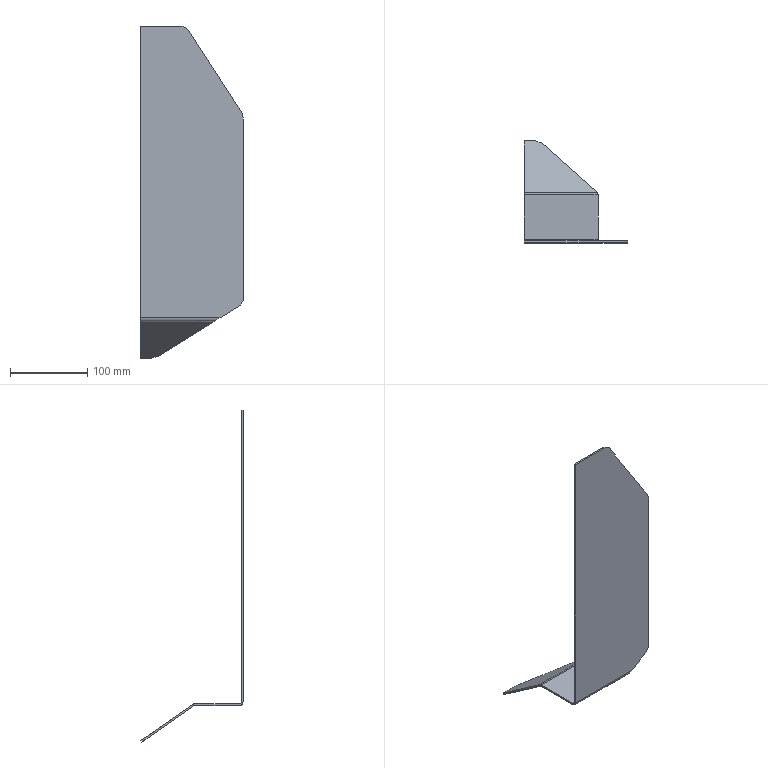Part | SolidWorks | features Chamfer 1, FlatPattern 1, ICE 1, SMBaseFlange 1, SheetMetal 1 | 1 solid | 28 faces | box 134 x 132 x 429.026 mm | volume 130634 mm3 | plane 22 | cylinder 4 | spline 2 | commonest cylinder face diameters 5 x2 9.6 x2
STEP:
#1=CARTESIAN_POINT('',(-52.,128.384,-429.026));
#2=VERTEX_POINT('',#1);
#3=CARTESIAN_POINT('',(-67.,128.384,-429.026));
#4=VERTEX_POINT('',#3);
#5=CARTESIAN_POINT('',(67.,128.384,-429.026));
#6=DIRECTION('',(-1.,0.,0.));
#7=VECTOR('',#6,1000.);
#8=LINE('',#5,#7);
#9=EDGE_CURVE('',#2,#4,#8,.T.);
#10=ORIENTED_EDGE('',*,*,#9,.F.);
#11=CARTESIAN_POINT('',(-43.618,125.364,-426.919));
#12=VERTEX_POINT('',#11);
#13=CARTESIAN_POINT('',(-43.618,125.364,-426.919));
#14=DIRECTION('',(0.9155,-0.3299,0.2302));
#15=VECTOR('',#14,1000.);
#16=LINE('',#13,#15);
#17=EDGE_CURVE('',#2,#12,#16,.T.);
#18=ORIENTED_EDGE('',*,*,#17,.T.);
#19=CARTESIAN_POINT('',(27.757,61.622,-382.45));
#20=VERTEX_POINT('',#19);
#21=CARTESIAN_POINT('',(46.463,44.916,-370.795));
#22=DIRECTION('',(0.6764,-0.6041,0.4214));
#23=VECTOR('',#22,1000.);
#24=LINE('',#21,#23);
#25=EDGE_CURVE('',#12,#20,#24,.T.);
#26=ORIENTED_EDGE('',*,*,#25,.T.);
#27=CARTESIAN_POINT('',(-67.,61.622,-382.45));
#28=VERTEX_POINT('',#27);
#29=CARTESIAN_POINT('',(67.,61.622,-382.45));
#30=DIRECTION('',(-1.,0.,0.));
#31=VECTOR('',#30,1000.);
#32=LINE('',#29,#31);
#33=EDGE_CURVE('',#20,#28,#32,.T.);
#34=ORIENTED_EDGE('',*,*,#33,.T.);
#35=CARTESIAN_POINT('',(-67.,60.384,-381.586));
#36=DIRECTION('',(0.,0.8201,-0.5722));
#37=VECTOR('',#36,1000.);
#38=LINE('',#35,#37);
#39=EDGE_CURVE('',#28,#4,#38,.T.);
#40=ORIENTED_EDGE('',*,*,#39,.T.);
#41=EDGE_LOOP('',(#10,#18,#26,#34,#40));
#42=FACE_OUTER_BOUND('',#41,.T.);
#43=CARTESIAN_POINT('',(67.,60.384,-381.586));
#44=DIRECTION('',(0.,0.5722,0.8201));
#45=DIRECTION('',(0.,-0.8201,0.5722));
#46=AXIS2_PLACEMENT_3D('',#43,#44,#45);
#47=PLANE('',#46);
#48=ADVANCED_FACE('',(#42),#47,.F.);
#49=CARTESIAN_POINT('',(-52.,129.7,-427.14));
#50=VERTEX_POINT('',#49);
#51=CARTESIAN_POINT('',(-67.,129.7,-427.14));
#52=VERTEX_POINT('',#51);
#53=CARTESIAN_POINT('',(67.,129.7,-427.14));
#54=DIRECTION('',(-1.,0.,0.));
#55=VECTOR('',#54,1000.);
#56=LINE('',#53,#55);
#57=EDGE_CURVE('',#50,#52,#56,.T.);
#58=ORIENTED_EDGE('',*,*,#57,.F.);
#59=CARTESIAN_POINT('',(-52.,129.7,-427.14));
#60=DIRECTION('',(0.,-0.5722,-0.8201));
#61=VECTOR('',#60,1000.);
#62=LINE('',#59,#61);
#63=EDGE_CURVE('',#50,#2,#62,.T.);
#64=ORIENTED_EDGE('',*,*,#63,.T.);
#65=ORIENTED_EDGE('',*,*,#9,.T.);
#66=CARTESIAN_POINT('',(-67.,129.7,-427.14));
#67=DIRECTION('',(0.,-0.5722,-0.8201));
#68=VECTOR('',#67,1000.);
#69=LINE('',#66,#68);
#70=EDGE_CURVE('',#52,#4,#69,.T.);
#71=ORIENTED_EDGE('',*,*,#70,.F.);
#72=EDGE_LOOP('',(#58,#64,#65,#71));
#73=FACE_OUTER_BOUND('',#72,.T.);
#74=CARTESIAN_POINT('',(67.,129.7,-427.14));
#75=DIRECTION('',(0.,0.8201,-0.5722));
#76=DIRECTION('',(0.,0.5722,0.8201));
#77=AXIS2_PLACEMENT_3D('',#74,#75,#76);
#78=PLANE('',#77);
#79=ADVANCED_FACE('',(#73),#78,.T.);
#80=CARTESIAN_POINT('',(-43.618,126.68,-425.033));
#81=VERTEX_POINT('',#80);
#82=CARTESIAN_POINT('',(27.757,62.938,-380.563));
#83=VERTEX_POINT('',#82);
#84=CARTESIAN_POINT('',(46.463,46.232,-368.909));
#85=DIRECTION('',(0.6764,-0.6041,0.4214));
#86=VECTOR('',#85,1000.);
#87=LINE('',#84,#86);
#88=EDGE_CURVE('',#81,#83,#87,.T.);
#89=ORIENTED_EDGE('',*,*,#88,.F.);
#90=CARTESIAN_POINT('',(78.28,82.756,-394.39));
#91=DIRECTION('',(-0.9155,0.3299,-0.2302));
#92=VECTOR('',#91,1000.);
#93=LINE('',#90,#92);
#94=EDGE_CURVE('',#81,#50,#93,.T.);
#95=ORIENTED_EDGE('',*,*,#94,.T.);
#96=ORIENTED_EDGE('',*,*,#57,.T.);
#97=CARTESIAN_POINT('',(-67.,62.938,-380.563));
#98=VERTEX_POINT('',#97);
#99=CARTESIAN_POINT('',(-67.,61.7,-379.7));
#100=DIRECTION('',(0.,0.8201,-0.5722));
#101=VECTOR('',#100,1000.);
#102=LINE('',#99,#101);
#103=EDGE_CURVE('',#98,#52,#102,.T.);
#104=ORIENTED_EDGE('',*,*,#103,.F.);
#105=CARTESIAN_POINT('',(67.,62.938,-380.563));
#106=DIRECTION('',(-1.,0.,0.));
#107=VECTOR('',#106,1000.);
#108=LINE('',#105,#107);
#109=EDGE_CURVE('',#83,#98,#108,.T.);
#110=ORIENTED_EDGE('',*,*,#109,.F.);
#111=EDGE_LOOP('',(#89,#95,#96,#104,#110));
#112=FACE_OUTER_BOUND('',#111,.T.);
#113=CARTESIAN_POINT('',(67.,61.7,-379.7));
#114=DIRECTION('',(0.,0.5722,0.8201));
#115=DIRECTION('',(0.,-0.8201,0.5722));
#116=AXIS2_PLACEMENT_3D('',#113,#114,#115);
#117=PLANE('',#116);
#118=ADVANCED_FACE('',(#112),#117,.T.);
#119=CARTESIAN_POINT('',(28.479,60.191,-379.7));
#120=VERTEX_POINT('',#119);
#121=CARTESIAN_POINT('',(-67.,60.191,-379.7));
#122=VERTEX_POINT('',#121);
#123=CARTESIAN_POINT('',(67.,60.191,-379.7));
#124=DIRECTION('',(-1.,0.,0.));
#125=VECTOR('',#124,1000.);
#126=LINE('',#123,#125);
#127=EDGE_CURVE('',#120,#122,#126,.T.);
#128=ORIENTED_EDGE('',*,*,#127,.F.);
#129=CARTESIAN_POINT('',(27.757,62.938,-380.563));
#130=CARTESIAN_POINT('',(28.231,62.126,-379.997));
#131=CARTESIAN_POINT('',(28.479,61.181,-379.7));
#132=CARTESIAN_POINT('',(28.479,60.191,-379.7));
#133=(BOUNDED_CURVE()B_SPLINE_CURVE(3,(#129,#130,#131,#132),.UNSPECIFIED.,.F.,.F.)B_SPLINE_CURVE_WITH_KNOTS((4,4),(2.532,3.142),.UNSPECIFIED.)CURVE()GEOMETRIC_REPRESENTATION_ITEM()RATIONAL_B_SPLINE_CURVE((1.,0.9693,0.9693,1.))REPRESENTATION_ITEM(''));
#134=EDGE_CURVE('',#83,#120,#133,.T.);
#135=ORIENTED_EDGE('',*,*,#134,.F.);
#136=ORIENTED_EDGE('',*,*,#109,.T.);
#137=CARTESIAN_POINT('',(-67.,60.191,-384.5));
#138=DIRECTION('',(-1.,0.,0.));
#139=DIRECTION('',(0.,0.,-1.));
#140=AXIS2_PLACEMENT_3D('',#137,#138,#139);
#141=CIRCLE('',#140,4.8);
#142=EDGE_CURVE('',#122,#98,#141,.T.);
#143=ORIENTED_EDGE('',*,*,#142,.F.);
#144=EDGE_LOOP('',(#128,#135,#136,#143));
#145=FACE_OUTER_BOUND('',#144,.T.);
#146=CARTESIAN_POINT('',(67.,60.191,-384.5));
#147=DIRECTION('',(-1.,0.,0.));
#148=DIRECTION('',(0.,0.,1.));
#149=AXIS2_PLACEMENT_3D('',#146,#147,#148);
#150=CYLINDRICAL_SURFACE('',#149,4.8);
#151=ADVANCED_FACE('',(#145),#150,.T.);
#152=CARTESIAN_POINT('',(28.479,2.5,-379.7));
#153=VERTEX_POINT('',#152);
#154=CARTESIAN_POINT('',(-67.,2.5,-379.7));
#155=VERTEX_POINT('',#154);
#156=CARTESIAN_POINT('',(67.,2.5,-379.7));
#157=DIRECTION('',(-1.,0.,0.));
#158=VECTOR('',#157,1000.);
#159=LINE('',#156,#158);
#160=EDGE_CURVE('',#153,#155,#159,.T.);
#161=ORIENTED_EDGE('',*,*,#160,.F.);
#162=CARTESIAN_POINT('',(28.479,0.,-379.7));
#163=DIRECTION('',(0.,-1.,0.));
#164=VECTOR('',#163,1000.);
#165=LINE('',#162,#164);
#166=EDGE_CURVE('',#120,#153,#165,.T.);
#167=ORIENTED_EDGE('',*,*,#166,.F.);
#168=ORIENTED_EDGE('',*,*,#127,.T.);
#169=CARTESIAN_POINT('',(-67.,0.,-379.7));
#170=DIRECTION('',(0.,1.,0.));
#171=VECTOR('',#170,1000.);
#172=LINE('',#169,#171);
#173=EDGE_CURVE('',#155,#122,#172,.T.);
#174=ORIENTED_EDGE('',*,*,#173,.F.);
#175=EDGE_LOOP('',(#161,#167,#168,#174));
#176=FACE_OUTER_BOUND('',#175,.T.);
#177=CARTESIAN_POINT('',(67.,0.,-379.7));
#178=DIRECTION('',(0.,0.,1.));
#179=DIRECTION('',(1.,0.,0.));
#180=AXIS2_PLACEMENT_3D('',#177,#178,#179);
#181=PLANE('',#180);
#182=ADVANCED_FACE('',(#176),#181,.T.);
#183=CARTESIAN_POINT('',(36.183,0.,-377.2));
#184=VERTEX_POINT('',#183);
#185=CARTESIAN_POINT('',(-67.,0.,-377.2));
#186=VERTEX_POINT('',#185);
#187=CARTESIAN_POINT('',(67.,0.,-377.2));
#188=DIRECTION('',(-1.,0.,0.));
#189=VECTOR('',#188,1000.);
#190=LINE('',#187,#189);
#191=EDGE_CURVE('',#184,#186,#190,.T.);
#192=ORIENTED_EDGE('',*,*,#191,.F.);
#193=CARTESIAN_POINT('',(28.479,2.5,-379.7));
#194=CARTESIAN_POINT('',(28.479,1.036,-379.7));
#195=CARTESIAN_POINT('',(31.67,0.,-378.664));
#196=CARTESIAN_POINT('',(36.183,0.,-377.2));
#197=(BOUNDED_CURVE()B_SPLINE_CURVE(3,(#193,#194,#195,#196),.UNSPECIFIED.,.F.,.T.)B_SPLINE_CURVE_WITH_KNOTS((4,4),(0.,1.571),.UNSPECIFIED.)CURVE()GEOMETRIC_REPRESENTATION_ITEM()RATIONAL_B_SPLINE_CURVE((1.,0.8047,0.8047,1.))REPRESENTATION_ITEM(''));
#198=EDGE_CURVE('',#153,#184,#197,.T.);
#199=ORIENTED_EDGE('',*,*,#198,.F.);
#200=ORIENTED_EDGE('',*,*,#160,.T.);
#201=CARTESIAN_POINT('',(-67.,2.5,-377.2));
#202=DIRECTION('',(1.,0.,0.));
#203=DIRECTION('',(0.,0.,1.));
#204=AXIS2_PLACEMENT_3D('',#201,#202,#203);
#205=CIRCLE('',#204,2.5);
#206=EDGE_CURVE('',#186,#155,#205,.T.);
#207=ORIENTED_EDGE('',*,*,#206,.F.);
#208=EDGE_LOOP('',(#192,#199,#200,#207));
#209=FACE_OUTER_BOUND('',#208,.T.);
#210=CARTESIAN_POINT('',(67.,2.5,-377.2));
#211=DIRECTION('',(-1.,0.,0.));
#212=DIRECTION('',(0.,0.,1.));
#213=AXIS2_PLACEMENT_3D('',#210,#211,#212);
#214=CYLINDRICAL_SURFACE('',#213,2.5);
#215=ADVANCED_FACE('',(#209),#214,.F.);
#216=CARTESIAN_POINT('',(67.,0.,-121.5));
#217=VERTEX_POINT('',#216);
#218=CARTESIAN_POINT('',(67.,0.,-353.));
#219=VERTEX_POINT('',#218);
#220=CARTESIAN_POINT('',(67.,0.,0.));
#221=DIRECTION('',(0.,0.,-1.));
#222=VECTOR('',#221,1000.);
#223=LINE('',#220,#222);
#224=EDGE_CURVE('',#217,#219,#223,.T.);
#225=ORIENTED_EDGE('',*,*,#224,.T.);
#226=CARTESIAN_POINT('',(62.756,0.,-360.644));
#227=VERTEX_POINT('',#226);
#228=CARTESIAN_POINT('',(216.804,0.,-83.167));
#229=DIRECTION('',(-0.4854,0.,-0.8743));
#230=VECTOR('',#229,1000.);
#231=LINE('',#228,#230);
#232=EDGE_CURVE('',#219,#227,#231,.T.);
#233=ORIENTED_EDGE('',*,*,#232,.T.);
#234=CARTESIAN_POINT('',(227.677,0.,-257.892));
#235=DIRECTION('',(0.8487,0.,0.5288));
#236=VECTOR('',#235,1000.);
#237=LINE('',#234,#236);
#238=EDGE_CURVE('',#184,#227,#237,.T.);
#239=ORIENTED_EDGE('',*,*,#238,.F.);
#240=ORIENTED_EDGE('',*,*,#191,.T.);
#241=CARTESIAN_POINT('',(-67.,0.,0.));
#242=VERTEX_POINT('',#241);
#243=CARTESIAN_POINT('',(-67.,0.,0.));
#244=DIRECTION('',(0.,0.,-1.));
#245=VECTOR('',#244,1000.);
#246=LINE('',#243,#245);
#247=EDGE_CURVE('',#242,#186,#246,.T.);
#248=ORIENTED_EDGE('',*,*,#247,.F.);
#249=CARTESIAN_POINT('',(-13.,0.,0.));
#250=VERTEX_POINT('',#249);
#251=CARTESIAN_POINT('',(67.,0.,0.));
#252=DIRECTION('',(-1.,0.,0.));
#253=VECTOR('',#252,1000.);
#254=LINE('',#251,#253);
#255=EDGE_CURVE('',#250,#242,#254,.T.);
#256=ORIENTED_EDGE('',*,*,#255,.F.);
#257=CARTESIAN_POINT('',(-5.293,0.,-4.204));
#258=VERTEX_POINT('',#257);
#259=CARTESIAN_POINT('',(48.652,0.,-33.633));
#260=DIRECTION('',(0.8779,0.,-0.4789));
#261=VECTOR('',#260,1000.);
#262=LINE('',#259,#261);
#263=EDGE_CURVE('',#250,#258,#262,.T.);
#264=ORIENTED_EDGE('',*,*,#263,.T.);
#265=CARTESIAN_POINT('',(64.293,0.,-112.296));
#266=VERTEX_POINT('',#265);
#267=CARTESIAN_POINT('',(13.976,0.,-34.136));
#268=DIRECTION('',(-0.5413,0.,0.8408));
#269=VECTOR('',#268,1000.);
#270=LINE('',#267,#269);
#271=EDGE_CURVE('',#266,#258,#270,.T.);
#272=ORIENTED_EDGE('',*,*,#271,.F.);
#273=CARTESIAN_POINT('',(34.116,0.,-9.67));
#274=DIRECTION('',(0.2821,0.,-0.9594));
#275=VECTOR('',#274,1000.);
#276=LINE('',#273,#275);
#277=EDGE_CURVE('',#266,#217,#276,.T.);
#278=ORIENTED_EDGE('',*,*,#277,.T.);
#279=EDGE_LOOP('',(#225,#233,#239,#240,#248,#256,#264,#272,#278));
#280=FACE_OUTER_BOUND('',#279,.T.);
#281=CARTESIAN_POINT('',(67.,0.,0.));
#282=DIRECTION('',(0.,1.,0.));
#283=DIRECTION('',(0.,0.,1.));
#284=AXIS2_PLACEMENT_3D('',#281,#282,#283);
#285=PLANE('',#284);
#286=ADVANCED_FACE('',(#280),#285,.T.);
#287=CARTESIAN_POINT('',(-13.,-2.3,0.));
#288=VERTEX_POINT('',#287);
#289=CARTESIAN_POINT('',(-67.,-2.3,0.));
#290=VERTEX_POINT('',#289);
#291=CARTESIAN_POINT('',(67.,-2.3,0.));
#292=DIRECTION('',(-1.,0.,0.));
#293=VECTOR('',#292,1000.);
#294=LINE('',#291,#293);
#295=EDGE_CURVE('',#288,#290,#294,.T.);
#296=ORIENTED_EDGE('',*,*,#295,.F.);
#297=CARTESIAN_POINT('',(-13.,-2.3,0.));
#298=DIRECTION('',(0.,1.,0.));
#299=VECTOR('',#298,1000.);
#300=LINE('',#297,#299);
#301=EDGE_CURVE('',#288,#250,#300,.T.);
#302=ORIENTED_EDGE('',*,*,#301,.T.);
#303=ORIENTED_EDGE('',*,*,#255,.T.);
#304=CARTESIAN_POINT('',(-67.,-2.3,0.));
#305=DIRECTION('',(0.,1.,0.));
#306=VECTOR('',#305,1000.);
#307=LINE('',#304,#306);
#308=EDGE_CURVE('',#290,#242,#307,.T.);
#309=ORIENTED_EDGE('',*,*,#308,.F.);
#310=EDGE_LOOP('',(#296,#302,#303,#309));
#311=FACE_OUTER_BOUND('',#310,.T.);
#312=CARTESIAN_POINT('',(67.,-2.3,0.));
#313=DIRECTION('',(0.,0.,1.));
#314=DIRECTION('',(1.,0.,0.));
#315=AXIS2_PLACEMENT_3D('',#312,#313,#314);
#316=PLANE('',#315);
#317=ADVANCED_FACE('',(#311),#316,.T.);
#318=CARTESIAN_POINT('',(36.183,-2.3,-377.2));
#319=VERTEX_POINT('',#318);
#320=CARTESIAN_POINT('',(62.756,-2.3,-360.644));
#321=VERTEX_POINT('',#320);
#322=CARTESIAN_POINT('',(227.677,-2.3,-257.892));
#323=DIRECTION('',(0.8487,0.,0.5288));
#324=VECTOR('',#323,1000.);
#325=LINE('',#322,#324);
#326=EDGE_CURVE('',#319,#321,#325,.T.);
#327=ORIENTED_EDGE('',*,*,#326,.T.);
#328=CARTESIAN_POINT('',(67.,-2.3,-353.));
#329=VERTEX_POINT('',#328);
#330=CARTESIAN_POINT('',(62.756,-2.3,-360.644));
#331=DIRECTION('',(0.4854,0.,0.8743));
#332=VECTOR('',#331,1000.);
#333=LINE('',#330,#332);
#334=EDGE_CURVE('',#321,#329,#333,.T.);
#335=ORIENTED_EDGE('',*,*,#334,.T.);
#336=CARTESIAN_POINT('',(67.,-2.3,-121.5));
#337=VERTEX_POINT('',#336);
#338=CARTESIAN_POINT('',(67.,-2.3,0.));
#339=DIRECTION('',(0.,0.,-1.));
#340=VECTOR('',#339,1000.);
#341=LINE('',#338,#340);
#342=EDGE_CURVE('',#337,#329,#341,.T.);
#343=ORIENTED_EDGE('',*,*,#342,.F.);
#344=CARTESIAN_POINT('',(64.293,-2.3,-112.296));
#345=VERTEX_POINT('',#344);
#346=CARTESIAN_POINT('',(67.,-2.3,-121.5));
#347=DIRECTION('',(-0.2821,0.,0.9594));
#348=VECTOR('',#347,1000.);
#349=LINE('',#346,#348);
#350=EDGE_CURVE('',#337,#345,#349,.T.);
#351=ORIENTED_EDGE('',*,*,#350,.T.);
#352=CARTESIAN_POINT('',(-5.293,-2.3,-4.204));
#353=VERTEX_POINT('',#352);
#354=CARTESIAN_POINT('',(13.976,-2.3,-34.136));
#355=DIRECTION('',(-0.5413,0.,0.8408));
#356=VECTOR('',#355,1000.);
#357=LINE('',#354,#356);
#358=EDGE_CURVE('',#345,#353,#357,.T.);
#359=ORIENTED_EDGE('',*,*,#358,.T.);
#360=CARTESIAN_POINT('',(-5.293,-2.3,-4.204));
#361=DIRECTION('',(-0.8779,0.,0.4789));
#362=VECTOR('',#361,1000.);
#363=LINE('',#360,#362);
#364=EDGE_CURVE('',#353,#288,#363,.T.);
#365=ORIENTED_EDGE('',*,*,#364,.T.);
#366=ORIENTED_EDGE('',*,*,#295,.T.);
#367=CARTESIAN_POINT('',(-67.,-2.3,-377.2));
#368=VERTEX_POINT('',#367);
#369=CARTESIAN_POINT('',(-67.,-2.3,0.));
#370=DIRECTION('',(0.,0.,-1.));
#371=VECTOR('',#370,1000.);
#372=LINE('',#369,#371);
#373=EDGE_CURVE('',#290,#368,#372,.T.);
#374=ORIENTED_EDGE('',*,*,#373,.T.);
#375=CARTESIAN_POINT('',(67.,-2.3,-377.2));
#376=DIRECTION('',(-1.,0.,0.));
#377=VECTOR('',#376,1000.);
#378=LINE('',#375,#377);
#379=EDGE_CURVE('',#319,#368,#378,.T.);
#380=ORIENTED_EDGE('',*,*,#379,.F.);
#381=EDGE_LOOP('',(#327,#335,#343,#351,#359,#365,#366,#374,#380));
#382=FACE_OUTER_BOUND('',#381,.T.);
#383=CARTESIAN_POINT('',(67.,-2.3,0.));
#384=DIRECTION('',(0.,1.,0.));
#385=DIRECTION('',(0.,0.,1.));
#386=AXIS2_PLACEMENT_3D('',#383,#384,#385);
#387=PLANE('',#386);
#388=ADVANCED_FACE('',(#382),#387,.F.);
#389=CARTESIAN_POINT('',(28.479,2.5,-382.));
#390=VERTEX_POINT('',#389);
#391=CARTESIAN_POINT('',(28.479,2.5,-382.));
#392=CARTESIAN_POINT('',(28.479,-0.3118,-382.));
#393=CARTESIAN_POINT('',(31.67,-2.3,-380.012));
#394=CARTESIAN_POINT('',(36.183,-2.3,-377.2));
#395=(BOUNDED_CURVE()B_SPLINE_CURVE(3,(#391,#392,#393,#394),.UNSPECIFIED.,.F.,.F.)B_SPLINE_CURVE_WITH_KNOTS((4,4),(0.,1.571),.UNSPECIFIED.)CURVE()GEOMETRIC_REPRESENTATION_ITEM()RATIONAL_B_SPLINE_CURVE((1.,0.8047,0.8047,1.))REPRESENTATION_ITEM(''));
#396=EDGE_CURVE('',#390,#319,#395,.T.);
#397=ORIENTED_EDGE('',*,*,#396,.T.);
#398=ORIENTED_EDGE('',*,*,#379,.T.);
#399=CARTESIAN_POINT('',(-67.,2.5,-382.));
#400=VERTEX_POINT('',#399);
#401=CARTESIAN_POINT('',(-67.,2.5,-377.2));
#402=DIRECTION('',(1.,0.,0.));
#403=DIRECTION('',(0.,0.,-1.));
#404=AXIS2_PLACEMENT_3D('',#401,#402,#403);
#405=CIRCLE('',#404,4.8);
#406=EDGE_CURVE('',#368,#400,#405,.T.);
#407=ORIENTED_EDGE('',*,*,#406,.T.);
#408=CARTESIAN_POINT('',(67.,2.5,-382.));
#409=DIRECTION('',(-1.,0.,0.));
#410=VECTOR('',#409,1000.);
#411=LINE('',#408,#410);
#412=EDGE_CURVE('',#390,#400,#411,.T.);
#413=ORIENTED_EDGE('',*,*,#412,.F.);
#414=EDGE_LOOP('',(#397,#398,#407,#413));
#415=FACE_OUTER_BOUND('',#414,.T.);
#416=CARTESIAN_POINT('',(67.,2.5,-377.2));
#417=DIRECTION('',(-1.,0.,0.));
#418=DIRECTION('',(0.,0.,1.));
#419=AXIS2_PLACEMENT_3D('',#416,#417,#418);
#420=CYLINDRICAL_SURFACE('',#419,4.8);
#421=ADVANCED_FACE('',(#415),#420,.T.);
#422=CARTESIAN_POINT('',(28.479,60.191,-382.));
#423=VERTEX_POINT('',#422);
#424=CARTESIAN_POINT('',(28.479,0.,-382.));
#425=DIRECTION('',(0.,-1.,0.));
#426=VECTOR('',#425,1000.);
#427=LINE('',#424,#426);
#428=EDGE_CURVE('',#423,#390,#427,.T.);
#429=ORIENTED_EDGE('',*,*,#428,.T.);
#430=ORIENTED_EDGE('',*,*,#412,.T.);
#431=CARTESIAN_POINT('',(-67.,60.191,-382.));
#432=VERTEX_POINT('',#431);
#433=CARTESIAN_POINT('',(-67.,0.,-382.));
#434=DIRECTION('',(0.,1.,0.));
#435=VECTOR('',#434,1000.);
#436=LINE('',#433,#435);
#437=EDGE_CURVE('',#400,#432,#436,.T.);
#438=ORIENTED_EDGE('',*,*,#437,.T.);
#439=CARTESIAN_POINT('',(67.,60.191,-382.));
#440=DIRECTION('',(-1.,0.,0.));
#441=VECTOR('',#440,1000.);
#442=LINE('',#439,#441);
#443=EDGE_CURVE('',#423,#432,#442,.T.);
#444=ORIENTED_EDGE('',*,*,#443,.F.);
#445=EDGE_LOOP('',(#429,#430,#438,#444));
#446=FACE_OUTER_BOUND('',#445,.T.);
#447=CARTESIAN_POINT('',(67.,0.,-382.));
#448=DIRECTION('',(0.,0.,1.));
#449=DIRECTION('',(1.,0.,0.));
#450=AXIS2_PLACEMENT_3D('',#447,#448,#449);
#451=PLANE('',#450);
#452=ADVANCED_FACE('',(#446),#451,.F.);
#453=CARTESIAN_POINT('',(27.757,61.622,-382.45));
#454=CARTESIAN_POINT('',(28.231,61.199,-382.155));
#455=CARTESIAN_POINT('',(28.479,60.707,-382.));
#456=CARTESIAN_POINT('',(28.479,60.191,-382.));
#457=(BOUNDED_CURVE()B_SPLINE_CURVE(3,(#453,#454,#455,#456),.UNSPECIFIED.,.F.,.T.)B_SPLINE_CURVE_WITH_KNOTS((4,4),(2.532,3.142),.UNSPECIFIED.)CURVE()GEOMETRIC_REPRESENTATION_ITEM()RATIONAL_B_SPLINE_CURVE((1.,0.9693,0.9693,1.))REPRESENTATION_ITEM(''));
#458=EDGE_CURVE('',#20,#423,#457,.T.);
#459=ORIENTED_EDGE('',*,*,#458,.T.);
#460=ORIENTED_EDGE('',*,*,#443,.T.);
#461=CARTESIAN_POINT('',(-67.,60.191,-384.5));
#462=DIRECTION('',(-1.,0.,0.));
#463=DIRECTION('',(0.,0.,-1.));
#464=AXIS2_PLACEMENT_3D('',#461,#462,#463);
#465=CIRCLE('',#464,2.5);
#466=EDGE_CURVE('',#432,#28,#465,.T.);
#467=ORIENTED_EDGE('',*,*,#466,.T.);
#468=ORIENTED_EDGE('',*,*,#33,.F.);
#469=EDGE_LOOP('',(#459,#460,#467,#468));
#470=FACE_OUTER_BOUND('',#469,.T.);
#471=CARTESIAN_POINT('',(67.,60.191,-384.5));
#472=DIRECTION('',(-1.,0.,0.));
#473=DIRECTION('',(0.,0.,1.));
#474=AXIS2_PLACEMENT_3D('',#471,#472,#473);
#475=CYLINDRICAL_SURFACE('',#474,2.5);
#476=ADVANCED_FACE('',(#470),#475,.F.);
#477=ORIENTED_EDGE('',*,*,#342,.T.);
#478=CARTESIAN_POINT('',(67.,60.191,-353.));
#479=DIRECTION('',(0.,1.,0.));
#480=VECTOR('',#479,1000.);
#481=LINE('',#478,#480);
#482=EDGE_CURVE('',#329,#219,#481,.T.);
#483=ORIENTED_EDGE('',*,*,#482,.T.);
#484=ORIENTED_EDGE('',*,*,#224,.F.);
#485=CARTESIAN_POINT('',(67.,60.191,-121.5));
#486=DIRECTION('',(0.,-1.,0.));
#487=VECTOR('',#486,1000.);
#488=LINE('',#485,#487);
#489=EDGE_CURVE('',#217,#337,#488,.T.);
#490=ORIENTED_EDGE('',*,*,#489,.T.);
#491=EDGE_LOOP('',(#477,#483,#484,#490));
#492=FACE_OUTER_BOUND('',#491,.T.);
#493=CARTESIAN_POINT('',(67.,60.191,-384.5));
#494=DIRECTION('',(1.,0.,0.));
#495=DIRECTION('',(0.,0.,-1.));
#496=AXIS2_PLACEMENT_3D('',#493,#494,#495);
#497=PLANE('',#496);
#498=ADVANCED_FACE('',(#492),#497,.T.);
#499=CARTESIAN_POINT('',(-67.,0.,-377.2));
#500=DIRECTION('',(0.,-1.,0.));
#501=VECTOR('',#500,1000.);
#502=LINE('',#499,#501);
#503=EDGE_CURVE('',#186,#368,#502,.T.);
#504=ORIENTED_EDGE('',*,*,#503,.F.);
#505=ORIENTED_EDGE('',*,*,#206,.T.);
#506=CARTESIAN_POINT('',(-67.,2.5,-382.));
#507=DIRECTION('',(0.,0.,1.));
#508=VECTOR('',#507,1000.);
#509=LINE('',#506,#508);
#510=EDGE_CURVE('',#400,#155,#509,.T.);
#511=ORIENTED_EDGE('',*,*,#510,.F.);
#512=ORIENTED_EDGE('',*,*,#406,.F.);
#513=EDGE_LOOP('',(#504,#505,#511,#512));
#514=FACE_OUTER_BOUND('',#513,.T.);
#515=CARTESIAN_POINT('',(-67.,0.,-377.2));
#516=DIRECTION('',(-1.,0.,0.));
#517=DIRECTION('',(0.,0.,1.));
#518=AXIS2_PLACEMENT_3D('',#515,#516,#517);
#519=PLANE('',#518);
#520=ADVANCED_FACE('',(#514),#519,.T.);
#521=ORIENTED_EDGE('',*,*,#247,.T.);
#522=ORIENTED_EDGE('',*,*,#503,.T.);
#523=ORIENTED_EDGE('',*,*,#373,.F.);
#524=ORIENTED_EDGE('',*,*,#308,.T.);
#525=EDGE_LOOP('',(#521,#522,#523,#524));
#526=FACE_OUTER_BOUND('',#525,.T.);
#527=CARTESIAN_POINT('',(-67.,2.5,-382.));
#528=DIRECTION('',(-1.,0.,0.));
#529=DIRECTION('',(0.,0.,1.));
#530=AXIS2_PLACEMENT_3D('',#527,#528,#529);
#531=PLANE('',#530);
#532=ADVANCED_FACE('',(#526),#531,.T.);
#533=CARTESIAN_POINT('',(-67.,60.191,-379.7));
#534=DIRECTION('',(0.,0.,-1.));
#535=VECTOR('',#534,1000.);
#536=LINE('',#533,#535);
#537=EDGE_CURVE('',#122,#432,#536,.T.);
#538=ORIENTED_EDGE('',*,*,#537,.F.);
#539=ORIENTED_EDGE('',*,*,#142,.T.);
#540=CARTESIAN_POINT('',(-67.,61.622,-382.45));
#541=DIRECTION('',(0.,0.5722,0.8201));
#542=VECTOR('',#541,1000.);
#543=LINE('',#540,#542);
#544=EDGE_CURVE('',#28,#98,#543,.T.);
#545=ORIENTED_EDGE('',*,*,#544,.F.);
#546=ORIENTED_EDGE('',*,*,#466,.F.);
#547=EDGE_LOOP('',(#538,#539,#545,#546));
#548=FACE_OUTER_BOUND('',#547,.T.);
#549=CARTESIAN_POINT('',(-67.,60.191,-379.7));
#550=DIRECTION('',(-1.,0.,0.));
#551=DIRECTION('',(0.,0.,1.));
#552=AXIS2_PLACEMENT_3D('',#549,#550,#551);
#553=PLANE('',#552);
#554=ADVANCED_FACE('',(#548),#553,.T.);
#555=ORIENTED_EDGE('',*,*,#173,.T.);
#556=ORIENTED_EDGE('',*,*,#537,.T.);
#557=ORIENTED_EDGE('',*,*,#437,.F.);
#558=ORIENTED_EDGE('',*,*,#510,.T.);
#559=EDGE_LOOP('',(#555,#556,#557,#558));
#560=FACE_OUTER_BOUND('',#559,.T.);
#561=CARTESIAN_POINT('',(-67.,61.622,-382.45));
#562=DIRECTION('',(-1.,0.,0.));
#563=DIRECTION('',(0.,0.,1.));
#564=AXIS2_PLACEMENT_3D('',#561,#562,#563);
#565=PLANE('',#564);
#566=ADVANCED_FACE('',(#560),#565,.T.);
#567=ORIENTED_EDGE('',*,*,#39,.F.);
#568=ORIENTED_EDGE('',*,*,#544,.T.);
#569=ORIENTED_EDGE('',*,*,#103,.T.);
#570=ORIENTED_EDGE('',*,*,#70,.T.);
#571=EDGE_LOOP('',(#567,#568,#569,#570));
#572=FACE_OUTER_BOUND('',#571,.T.);
#573=CARTESIAN_POINT('',(-67.,60.191,-384.5));
#574=DIRECTION('',(1.,0.,0.));
#575=DIRECTION('',(0.,0.,-1.));
#576=AXIS2_PLACEMENT_3D('',#573,#574,#575);
#577=PLANE('',#576);
#578=ADVANCED_FACE('',(#572),#577,.F.);
#579=CARTESIAN_POINT('',(28.479,2.5,-382.));
#580=DIRECTION('',(0.,0.,1.));
#581=VECTOR('',#580,1000.);
#582=LINE('',#579,#581);
#583=EDGE_CURVE('',#390,#153,#582,.T.);
#584=ORIENTED_EDGE('',*,*,#583,.F.);
#585=ORIENTED_EDGE('',*,*,#428,.F.);
#586=CARTESIAN_POINT('',(28.479,60.191,-382.));
#587=DIRECTION('',(0.,0.,1.));
#588=VECTOR('',#587,1000.);
#589=LINE('',#586,#588);
#590=EDGE_CURVE('',#423,#120,#589,.T.);
#591=ORIENTED_EDGE('',*,*,#590,.T.);
#592=ORIENTED_EDGE('',*,*,#166,.T.);
#593=EDGE_LOOP('',(#584,#585,#591,#592));
#594=FACE_OUTER_BOUND('',#593,.T.);
#595=CARTESIAN_POINT('',(28.479,0.,-382.));
#596=DIRECTION('',(-1.,0.,0.));
#597=DIRECTION('',(0.,-1.,0.));
#598=AXIS2_PLACEMENT_3D('',#595,#596,#597);
#599=PLANE('',#598);
#600=ADVANCED_FACE('',(#594),#599,.F.);
#601=CARTESIAN_POINT('',(36.183,0.,-377.2));
#602=DIRECTION('',(0.,-1.,0.));
#603=VECTOR('',#602,1000.);
#604=LINE('',#601,#603);
#605=EDGE_CURVE('',#184,#319,#604,.T.);
#606=ORIENTED_EDGE('',*,*,#605,.T.);
#607=ORIENTED_EDGE('',*,*,#396,.F.);
#608=ORIENTED_EDGE('',*,*,#583,.T.);
#609=ORIENTED_EDGE('',*,*,#198,.T.);
#610=EDGE_LOOP('',(#606,#607,#608,#609));
#611=FACE_OUTER_BOUND('',#610,.T.);
#612=CARTESIAN_POINT('',(28.479,2.5,-379.7));
#613=CARTESIAN_POINT('',(28.479,2.5,-380.467));
#614=CARTESIAN_POINT('',(28.479,2.5,-381.233));
#615=CARTESIAN_POINT('',(28.479,2.5,-382.));
#616=CARTESIAN_POINT('',(28.479,-2.5,-379.7));
#617=CARTESIAN_POINT('',(28.479,-4.033,-380.467));
#618=CARTESIAN_POINT('',(28.479,-5.567,-381.233));
#619=CARTESIAN_POINT('',(28.479,-7.1,-382.));
#620=CARTESIAN_POINT('',(43.887,-2.5,-374.7));
#621=CARTESIAN_POINT('',(43.887,-4.033,-373.933));
#622=CARTESIAN_POINT('',(43.887,-5.567,-373.167));
#623=CARTESIAN_POINT('',(43.887,-7.1,-372.4));
#624=CARTESIAN_POINT('',(43.887,2.5,-374.7));
#625=CARTESIAN_POINT('',(43.887,2.5,-373.933));
#626=CARTESIAN_POINT('',(43.887,2.5,-373.167));
#627=CARTESIAN_POINT('',(43.887,2.5,-372.4));
#628=CARTESIAN_POINT('',(43.887,7.5,-374.7));
#629=CARTESIAN_POINT('',(43.887,9.033,-373.933));
#630=CARTESIAN_POINT('',(43.887,10.567,-373.167));
#631=CARTESIAN_POINT('',(43.887,12.1,-372.4));
#632=CARTESIAN_POINT('',(28.479,7.5,-379.7));
#633=CARTESIAN_POINT('',(28.479,9.033,-380.467));
#634=CARTESIAN_POINT('',(28.479,10.567,-381.233));
#635=CARTESIAN_POINT('',(28.479,12.1,-382.));
#636=CARTESIAN_POINT('',(28.479,2.5,-379.7));
#637=CARTESIAN_POINT('',(28.479,2.5,-380.467));
#638=CARTESIAN_POINT('',(28.479,2.5,-381.233));
#639=CARTESIAN_POINT('',(28.479,2.5,-382.));
#640=(BOUNDED_SURFACE()B_SPLINE_SURFACE(3,3,((#612,#613,#614,#615),(#616,#617,#618,#619),(#620,#621,#622,#623),(#624,#625,#626,#627),(#628,#629,#630,#631),(#632,#633,#634,#635),(#636,#637,#638,#639)),.UNSPECIFIED.,.T.,.F.,.T.)B_SPLINE_SURFACE_WITH_KNOTS((4,3,4),(4,4),(0.,0.5,1.),(0.,1.),.UNSPECIFIED.)GEOMETRIC_REPRESENTATION_ITEM()RATIONAL_B_SPLINE_SURFACE(((1.,1.,1.,1.),(0.3333,0.3333,0.3333,0.3333),(0.3333,0.3333,0.3333,0.3333),(1.,1.,1.,1.),(0.3333,0.3333,0.3333,0.3333),(0.3333,0.3333,0.3333,0.3333),(1.,1.,1.,1.)))REPRESENTATION_ITEM('')SURFACE());
#641=ADVANCED_FACE('',(#611),#640,.T.);
#642=ORIENTED_EDGE('',*,*,#238,.T.);
#643=CARTESIAN_POINT('',(62.756,0.,-360.644));
#644=DIRECTION('',(0.,-1.,0.));
#645=VECTOR('',#644,1000.);
#646=LINE('',#643,#645);
#647=EDGE_CURVE('',#227,#321,#646,.T.);
#648=ORIENTED_EDGE('',*,*,#647,.T.);
#649=ORIENTED_EDGE('',*,*,#326,.F.);
#650=ORIENTED_EDGE('',*,*,#605,.F.);
#651=EDGE_LOOP('',(#642,#648,#649,#650));
#652=FACE_OUTER_BOUND('',#651,.T.);
#653=CARTESIAN_POINT('',(227.677,0.,-257.892));
#654=DIRECTION('',(-0.5288,0.,0.8487));
#655=DIRECTION('',(0.8487,0.,0.5288));
#656=AXIS2_PLACEMENT_3D('',#653,#654,#655);
#657=PLANE('',#656);
#658=ADVANCED_FACE('',(#652),#657,.F.);
#659=ORIENTED_EDGE('',*,*,#590,.F.);
#660=ORIENTED_EDGE('',*,*,#458,.F.);
#661=CARTESIAN_POINT('',(27.757,61.622,-382.45));
#662=DIRECTION('',(0.,0.5722,0.8201));
#663=VECTOR('',#662,1000.);
#664=LINE('',#661,#663);
#665=EDGE_CURVE('',#20,#83,#664,.T.);
#666=ORIENTED_EDGE('',*,*,#665,.T.);
#667=ORIENTED_EDGE('',*,*,#134,.T.);
#668=EDGE_LOOP('',(#659,#660,#666,#667));
#669=FACE_OUTER_BOUND('',#668,.T.);
#670=CARTESIAN_POINT('',(20.454,60.191,-389.3));
#671=CARTESIAN_POINT('',(20.454,60.191,-388.533));
#672=CARTESIAN_POINT('',(20.454,60.191,-387.767));
#673=CARTESIAN_POINT('',(20.454,60.191,-387.));
#674=CARTESIAN_POINT('',(20.454,69.791,-389.3));
#675=CARTESIAN_POINT('',(20.454,68.258,-388.533));
#676=CARTESIAN_POINT('',(20.454,66.724,-387.767));
#677=CARTESIAN_POINT('',(20.454,65.191,-387.));
#678=CARTESIAN_POINT('',(28.479,69.791,-379.7));
#679=CARTESIAN_POINT('',(28.479,68.258,-380.467));
#680=CARTESIAN_POINT('',(28.479,66.724,-381.233));
#681=CARTESIAN_POINT('',(28.479,65.191,-382.));
#682=CARTESIAN_POINT('',(28.479,60.191,-379.7));
#683=CARTESIAN_POINT('',(28.479,60.191,-380.467));
#684=CARTESIAN_POINT('',(28.479,60.191,-381.233));
#685=CARTESIAN_POINT('',(28.479,60.191,-382.));
#686=CARTESIAN_POINT('',(28.479,50.591,-379.7));
#687=CARTESIAN_POINT('',(28.479,52.124,-380.467));
#688=CARTESIAN_POINT('',(28.479,53.658,-381.233));
#689=CARTESIAN_POINT('',(28.479,55.191,-382.));
#690=CARTESIAN_POINT('',(20.454,50.591,-389.3));
#691=CARTESIAN_POINT('',(20.454,52.124,-388.533));
#692=CARTESIAN_POINT('',(20.454,53.658,-387.767));
#693=CARTESIAN_POINT('',(20.454,55.191,-387.));
#694=CARTESIAN_POINT('',(20.454,60.191,-389.3));
#695=CARTESIAN_POINT('',(20.454,60.191,-388.533));
#696=CARTESIAN_POINT('',(20.454,60.191,-387.767));
#697=CARTESIAN_POINT('',(20.454,60.191,-387.));
#698=(BOUNDED_SURFACE()B_SPLINE_SURFACE(3,3,((#670,#671,#672,#673),(#674,#675,#676,#677),(#678,#679,#680,#681),(#682,#683,#684,#685),(#686,#687,#688,#689),(#690,#691,#692,#693),(#694,#695,#696,#697)),.UNSPECIFIED.,.T.,.F.,.T.)B_SPLINE_SURFACE_WITH_KNOTS((4,3,4),(4,4),(0.,0.5,1.),(0.,1.),.UNSPECIFIED.)GEOMETRIC_REPRESENTATION_ITEM()RATIONAL_B_SPLINE_SURFACE(((1.,1.,1.,1.),(0.3333,0.3333,0.3333,0.3333),(0.3333,0.3333,0.3333,0.3333),(1.,1.,1.,1.),(0.3333,0.3333,0.3333,0.3333),(0.3333,0.3333,0.3333,0.3333),(1.,1.,1.,1.)))REPRESENTATION_ITEM('')SURFACE());
#699=ADVANCED_FACE('',(#669),#698,.T.);
#700=ORIENTED_EDGE('',*,*,#25,.F.);
#701=CARTESIAN_POINT('',(-43.618,125.364,-426.919));
#702=DIRECTION('',(0.,0.5722,0.8201));
#703=VECTOR('',#702,1000.);
#704=LINE('',#701,#703);
#705=EDGE_CURVE('',#12,#81,#704,.T.);
#706=ORIENTED_EDGE('',*,*,#705,.T.);
#707=ORIENTED_EDGE('',*,*,#88,.T.);
#708=ORIENTED_EDGE('',*,*,#665,.F.);
#709=EDGE_LOOP('',(#700,#706,#707,#708));
#710=FACE_OUTER_BOUND('',#709,.T.);
#711=CARTESIAN_POINT('',(46.463,44.916,-370.795));
#712=DIRECTION('',(-0.7365,-0.5547,0.387));
#713=DIRECTION('',(0.6764,-0.6041,0.4214));
#714=AXIS2_PLACEMENT_3D('',#711,#712,#713);
#715=PLANE('',#714);
#716=ADVANCED_FACE('',(#710),#715,.F.);
#717=ORIENTED_EDGE('',*,*,#358,.F.);
#718=CARTESIAN_POINT('',(64.293,0.,-112.296));
#719=DIRECTION('',(0.,1.,0.));
#720=VECTOR('',#719,1000.);
#721=LINE('',#718,#720);
#722=EDGE_CURVE('',#345,#266,#721,.T.);
#723=ORIENTED_EDGE('',*,*,#722,.T.);
#724=ORIENTED_EDGE('',*,*,#271,.T.);
#725=CARTESIAN_POINT('',(-5.293,0.,-4.204));
#726=DIRECTION('',(0.,-1.,0.));
#727=VECTOR('',#726,1000.);
#728=LINE('',#725,#727);
#729=EDGE_CURVE('',#258,#353,#728,.T.);
#730=ORIENTED_EDGE('',*,*,#729,.T.);
#731=EDGE_LOOP('',(#717,#723,#724,#730));
#732=FACE_OUTER_BOUND('',#731,.T.);
#733=CARTESIAN_POINT('',(13.976,0.,-34.136));
#734=DIRECTION('',(-0.8408,0.,-0.5413));
#735=DIRECTION('',(-0.5413,0.,0.8408));
#736=AXIS2_PLACEMENT_3D('',#733,#734,#735);
#737=PLANE('',#736);
#738=ADVANCED_FACE('',(#732),#737,.F.);
#739=ORIENTED_EDGE('',*,*,#17,.F.);
#740=ORIENTED_EDGE('',*,*,#63,.F.);
#741=ORIENTED_EDGE('',*,*,#94,.F.);
#742=ORIENTED_EDGE('',*,*,#705,.F.);
#743=EDGE_LOOP('',(#739,#740,#741,#742));
#744=FACE_OUTER_BOUND('',#743,.T.);
#745=CARTESIAN_POINT('',(-43.618,125.364,-426.919));
#746=DIRECTION('',(0.4022,0.7509,-0.5238));
#747=DIRECTION('',(0.,-0.5722,-0.8201));
#748=AXIS2_PLACEMENT_3D('',#745,#746,#747);
#749=PLANE('',#748);
#750=ADVANCED_FACE('',(#744),#749,.T.);
#751=ORIENTED_EDGE('',*,*,#232,.F.);
#752=ORIENTED_EDGE('',*,*,#482,.F.);
#753=ORIENTED_EDGE('',*,*,#334,.F.);
#754=ORIENTED_EDGE('',*,*,#647,.F.);
#755=EDGE_LOOP('',(#751,#752,#753,#754));
#756=FACE_OUTER_BOUND('',#755,.T.);
#757=CARTESIAN_POINT('',(62.756,0.,-360.644));
#758=DIRECTION('',(0.8743,0.,-0.4854));
#759=DIRECTION('',(0.,1.,0.));
#760=AXIS2_PLACEMENT_3D('',#757,#758,#759);
#761=PLANE('',#760);
#762=ADVANCED_FACE('',(#756),#761,.T.);
#763=ORIENTED_EDGE('',*,*,#277,.F.);
#764=ORIENTED_EDGE('',*,*,#722,.F.);
#765=ORIENTED_EDGE('',*,*,#350,.F.);
#766=ORIENTED_EDGE('',*,*,#489,.F.);
#767=EDGE_LOOP('',(#763,#764,#765,#766));
#768=FACE_OUTER_BOUND('',#767,.T.);
#769=CARTESIAN_POINT('',(67.,60.191,-121.5));
#770=DIRECTION('',(0.9594,0.,0.2821));
#771=DIRECTION('',(0.,1.,0.));
#772=AXIS2_PLACEMENT_3D('',#769,#770,#771);
#773=PLANE('',#772);
#774=ADVANCED_FACE('',(#768),#773,.T.);
#775=ORIENTED_EDGE('',*,*,#263,.F.);
#776=ORIENTED_EDGE('',*,*,#301,.F.);
#777=ORIENTED_EDGE('',*,*,#364,.F.);
#778=ORIENTED_EDGE('',*,*,#729,.F.);
#779=EDGE_LOOP('',(#775,#776,#777,#778));
#780=FACE_OUTER_BOUND('',#779,.T.);
#781=CARTESIAN_POINT('',(-5.293,0.,-4.204));
#782=DIRECTION('',(0.4789,0.,0.8779));
#783=DIRECTION('',(0.,1.,0.));
#784=AXIS2_PLACEMENT_3D('',#781,#782,#783);
#785=PLANE('',#784);
#786=ADVANCED_FACE('',(#780),#785,.T.);
#787=CLOSED_SHELL('',(#48,#79,#118,#151,#182,#215,#286,#317,#388,#421,#452,#476,#498,#520,#532,#554,#566,#578,#600,#641,#658,#699,#716,#738,#750,#762,#774,#786));
#788=MANIFOLD_SOLID_BREP('',#787);
#789=CARTESIAN_POINT('',(0.,0.,0.));
#790=DIRECTION('',(0.,0.,1.));
#791=DIRECTION('',(1.,0.,0.));
#792=AXIS2_PLACEMENT_3D('',#789,#790,#791);
#793=(LENGTH_UNIT()NAMED_UNIT(*)SI_UNIT(.MILLI.,.METRE.));
#794=UNCERTAINTY_MEASURE_WITH_UNIT(LENGTH_MEASURE(0.00001),#793,'','');
#795=(NAMED_UNIT(*)PLANE_ANGLE_UNIT()SI_UNIT($,.RADIAN.));
#796=(NAMED_UNIT(*)SI_UNIT($,.STERADIAN.)SOLID_ANGLE_UNIT());
#797=(GEOMETRIC_REPRESENTATION_CONTEXT(3)GLOBAL_UNCERTAINTY_ASSIGNED_CONTEXT((#794))GLOBAL_UNIT_ASSIGNED_CONTEXT((#793,#795,#796))REPRESENTATION_CONTEXT('',''));
#798=ADVANCED_BREP_SHAPE_REPRESENTATION('',(#788,#792),#797);